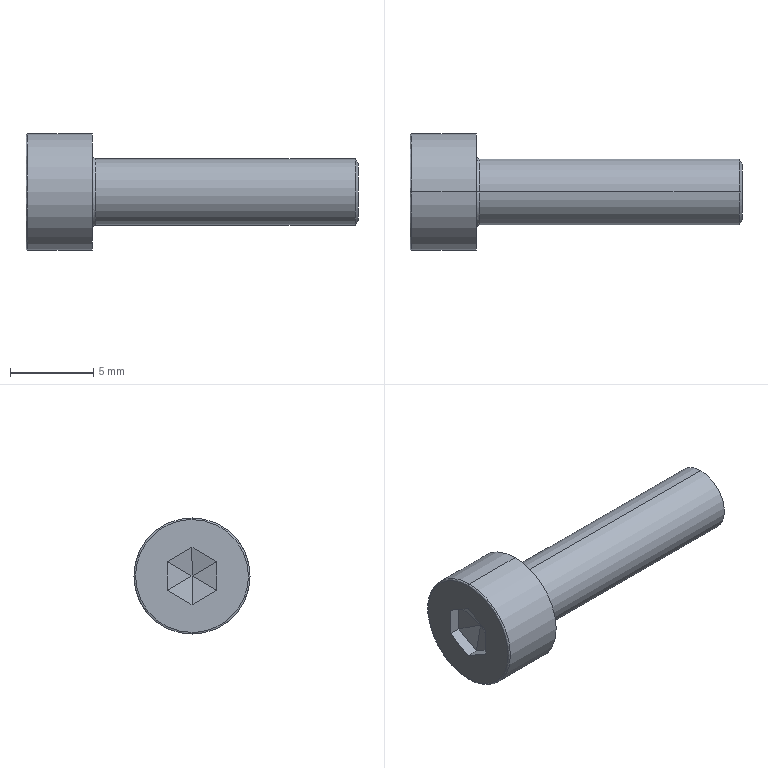Part | SolidWorks | features BaseBody 1 | 1 solid | 25 faces | box 20 x 7 x 7 mm | volume 348.346 mm3 | plane 15 | spline 4 | cylinder 4 | cone 2 | commonest cylinder face diameters 4 x2 7 x2
STEP:
#1=CARTESIAN_POINT('',(4.2,0.,-2.));
#2=VERTEX_POINT('',#1);
#3=CARTESIAN_POINT('',(4.2,0.,2.));
#4=VERTEX_POINT('',#3);
#5=CARTESIAN_POINT('',(4.2,0.,0.));
#6=DIRECTION('',(1.,0.,0.));
#7=DIRECTION('',(0.,0.,1.));
#8=AXIS2_PLACEMENT_3D('',#5,#6,#7);
#9=CIRCLE('',#8,2.);
#10=EDGE_CURVE('',#2,#4,#9,.T.);
#11=ORIENTED_EDGE('',*,*,#10,.F.);
#12=CARTESIAN_POINT('',(4.,0.,-2.2));
#13=VERTEX_POINT('',#12);
#14=CARTESIAN_POINT('',(4.2,0.,-2.2));
#15=DIRECTION('',(0.,-1.,0.));
#16=DIRECTION('',(0.,0.,-1.));
#17=AXIS2_PLACEMENT_3D('',#14,#15,#16);
#18=CIRCLE('',#17,0.2);
#19=EDGE_CURVE('',#2,#13,#18,.T.);
#20=ORIENTED_EDGE('',*,*,#19,.T.);
#21=CARTESIAN_POINT('',(4.,0.,2.2));
#22=VERTEX_POINT('',#21);
#23=CARTESIAN_POINT('',(4.,0.,2.2));
#24=CARTESIAN_POINT('',(4.,0.14,2.2));
#25=CARTESIAN_POINT('',(4.,0.3462,2.181));
#26=CARTESIAN_POINT('',(4.,0.5802,2.124));
#27=CARTESIAN_POINT('',(4.,0.6955,2.088));
#28=CARTESIAN_POINT('',(4.,0.7446,2.07));
#29=CARTESIAN_POINT('',(4.,0.7773,2.058));
#30=CARTESIAN_POINT('',(4.,0.7921,2.053));
#31=CARTESIAN_POINT('',(4.,1.093,1.934));
#32=CARTESIAN_POINT('',(4.,1.341,1.771));
#33=CARTESIAN_POINT('',(4.,1.663,1.448));
#34=CARTESIAN_POINT('',(4.,1.805,1.274));
#35=CARTESIAN_POINT('',(4.,1.937,1.049));
#36=CARTESIAN_POINT('',(4.,1.994,0.9314));
#37=CARTESIAN_POINT('',(4.,2.017,0.8797));
#38=CARTESIAN_POINT('',(4.,2.031,0.8449));
#39=CARTESIAN_POINT('',(4.,2.039,0.8261));
#40=CARTESIAN_POINT('',(4.,2.149,0.5493));
#41=CARTESIAN_POINT('',(4.,2.2,0.2801));
#42=CARTESIAN_POINT('',(4.,2.2,-0.1401));
#43=CARTESIAN_POINT('',(4.,2.181,-0.3463));
#44=CARTESIAN_POINT('',(4.,2.124,-0.5803));
#45=CARTESIAN_POINT('',(4.,2.088,-0.6956));
#46=CARTESIAN_POINT('',(4.,2.07,-0.7447));
#47=CARTESIAN_POINT('',(4.,2.058,-0.7773));
#48=CARTESIAN_POINT('',(4.,2.053,-0.7921));
#49=CARTESIAN_POINT('',(4.,1.934,-1.093));
#50=CARTESIAN_POINT('',(4.,1.771,-1.341));
#51=CARTESIAN_POINT('',(4.,1.448,-1.663));
#52=CARTESIAN_POINT('',(4.,1.274,-1.805));
#53=CARTESIAN_POINT('',(4.,1.049,-1.937));
#54=CARTESIAN_POINT('',(4.,0.9314,-1.994));
#55=CARTESIAN_POINT('',(4.,0.8797,-2.017));
#56=CARTESIAN_POINT('',(4.,0.8449,-2.031));
#57=CARTESIAN_POINT('',(4.,0.8261,-2.039));
#58=CARTESIAN_POINT('',(4.,0.5493,-2.149));
#59=CARTESIAN_POINT('',(4.,0.2801,-2.2));
#60=CARTESIAN_POINT('',(4.,0.,-2.2));
#61=B_SPLINE_CURVE_WITH_KNOTS('',3,(#23,#24,#25,#26,#27,#28,#29,#30,#31,#32,#33,#34,#35,#36,#37,#38,#39,#40,#41,#42,#43,#44,#45,#46,#47,#48,#49,#50,#51,#52,#53,#54,#55,#56,#57,#58,#59,#60),.UNSPECIFIED.,.F.,.F.,(4,1,1,1,2,2,2,1,1,1,2,2,2,1,1,1,2,2,2,1,1,1,2,2,4),(0.,0.03125,0.04688,0.05469,0.05859,0.0625,0.125,0.1563,0.1719,0.1797,0.1836,0.1875,0.25,0.2813,0.2969,0.3047,0.3086,0.3125,0.375,0.4062,0.4219,0.4297,0.4336,0.4375,0.5),.UNSPECIFIED.);
#62=EDGE_CURVE('',#22,#13,#61,.T.);
#63=ORIENTED_EDGE('',*,*,#62,.F.);
#64=CARTESIAN_POINT('',(4.2,0.,2.2));
#65=DIRECTION('',(0.,1.,0.));
#66=DIRECTION('',(0.,0.,1.));
#67=AXIS2_PLACEMENT_3D('',#64,#65,#66);
#68=CIRCLE('',#67,0.2);
#69=EDGE_CURVE('',#4,#22,#68,.T.);
#70=ORIENTED_EDGE('',*,*,#69,.F.);
#71=EDGE_LOOP('',(#11,#20,#63,#70));
#72=FACE_OUTER_BOUND('',#71,.T.);
#73=CARTESIAN_POINT('',(4.2,0.,2.));
#74=CARTESIAN_POINT('',(4.2,4.,2.));
#75=CARTESIAN_POINT('',(4.2,4.,-2.));
#76=CARTESIAN_POINT('',(4.2,0.,-2.));
#77=CARTESIAN_POINT('',(4.083,0.,2.));
#78=CARTESIAN_POINT('',(4.083,4.,2.));
#79=CARTESIAN_POINT('',(4.083,4.,-2.));
#80=CARTESIAN_POINT('',(4.083,0.,-2.));
#81=CARTESIAN_POINT('',(4.,0.,2.083));
#82=CARTESIAN_POINT('',(4.,4.166,2.083));
#83=CARTESIAN_POINT('',(4.,4.166,-2.083));
#84=CARTESIAN_POINT('',(4.,0.,-2.083));
#85=CARTESIAN_POINT('',(4.,0.,2.2));
#86=CARTESIAN_POINT('',(4.,4.4,2.2));
#87=CARTESIAN_POINT('',(4.,4.4,-2.2));
#88=CARTESIAN_POINT('',(4.,0.,-2.2));
#89=(BOUNDED_SURFACE()B_SPLINE_SURFACE(3,3,((#73,#74,#75,#76),(#77,#78,#79,#80),(#81,#82,#83,#84),(#85,#86,#87,#88)),.UNSPECIFIED.,.F.,.F.,.F.)B_SPLINE_SURFACE_WITH_KNOTS((4,4),(4,4),(0.,1.),(0.,1.),.UNSPECIFIED.)GEOMETRIC_REPRESENTATION_ITEM()RATIONAL_B_SPLINE_SURFACE(((1.,0.3333,0.3333,1.),(0.8047,0.2682,0.2682,0.8047),(0.8047,0.2682,0.2682,0.8047),(1.,0.3333,0.3333,1.)))REPRESENTATION_ITEM('')SURFACE());
#90=ADVANCED_FACE('',(#72),#89,.F.);
#91=CARTESIAN_POINT('',(0.1,0.,3.5));
#92=VERTEX_POINT('',#91);
#93=CARTESIAN_POINT('',(0.1,0.,-3.5));
#94=VERTEX_POINT('',#93);
#95=CARTESIAN_POINT('',(0.1,0.,0.));
#96=DIRECTION('',(1.,0.,0.));
#97=DIRECTION('',(0.,0.,1.));
#98=AXIS2_PLACEMENT_3D('',#95,#96,#97);
#99=CIRCLE('',#98,3.5);
#100=EDGE_CURVE('',#92,#94,#99,.T.);
#101=ORIENTED_EDGE('',*,*,#100,.F.);
#102=CARTESIAN_POINT('',(0.,0.,3.4));
#103=VERTEX_POINT('',#102);
#104=CARTESIAN_POINT('',(0.1,0.,3.4));
#105=DIRECTION('',(0.,-1.,0.));
#106=DIRECTION('',(0.,0.,1.));
#107=AXIS2_PLACEMENT_3D('',#104,#105,#106);
#108=CIRCLE('',#107,0.1);
#109=EDGE_CURVE('',#92,#103,#108,.T.);
#110=ORIENTED_EDGE('',*,*,#109,.T.);
#111=CARTESIAN_POINT('',(0.,0.,-3.4));
#112=VERTEX_POINT('',#111);
#113=CARTESIAN_POINT('',(0.,0.,3.4));
#114=CARTESIAN_POINT('',(0.,-6.8,3.4));
#115=CARTESIAN_POINT('',(0.,-6.8,-3.4));
#116=CARTESIAN_POINT('',(0.,0.,-3.4));
#117=(BOUNDED_CURVE()B_SPLINE_CURVE(3,(#113,#114,#115,#116),.UNSPECIFIED.,.F.,.F.)B_SPLINE_CURVE_WITH_KNOTS((4,4),(0.5,1.),.UNSPECIFIED.)CURVE()GEOMETRIC_REPRESENTATION_ITEM()RATIONAL_B_SPLINE_CURVE((1.,0.3333,0.3333,1.))REPRESENTATION_ITEM(''));
#118=EDGE_CURVE('',#103,#112,#117,.T.);
#119=ORIENTED_EDGE('',*,*,#118,.T.);
#120=CARTESIAN_POINT('',(0.1,0.,-3.4));
#121=DIRECTION('',(0.,1.,0.));
#122=DIRECTION('',(0.,0.,-1.));
#123=AXIS2_PLACEMENT_3D('',#120,#121,#122);
#124=CIRCLE('',#123,0.1);
#125=EDGE_CURVE('',#94,#112,#124,.T.);
#126=ORIENTED_EDGE('',*,*,#125,.F.);
#127=EDGE_LOOP('',(#101,#110,#119,#126));
#128=FACE_OUTER_BOUND('',#127,.T.);
#129=CARTESIAN_POINT('',(0.1,0.,3.5));
#130=CARTESIAN_POINT('',(0.1,-7.,3.5));
#131=CARTESIAN_POINT('',(0.1,-7.,-3.5));
#132=CARTESIAN_POINT('',(0.1,0.,-3.5));
#133=CARTESIAN_POINT('',(0.04142,0.,3.5));
#134=CARTESIAN_POINT('',(0.04142,-7.,3.5));
#135=CARTESIAN_POINT('',(0.04142,-7.,-3.5));
#136=CARTESIAN_POINT('',(0.04142,0.,-3.5));
#137=CARTESIAN_POINT('',(0.,0.,3.459));
#138=CARTESIAN_POINT('',(0.,-6.917,3.459));
#139=CARTESIAN_POINT('',(0.,-6.917,-3.459));
#140=CARTESIAN_POINT('',(0.,0.,-3.459));
#141=CARTESIAN_POINT('',(0.,0.,3.4));
#142=CARTESIAN_POINT('',(0.,-6.8,3.4));
#143=CARTESIAN_POINT('',(0.,-6.8,-3.4));
#144=CARTESIAN_POINT('',(0.,0.,-3.4));
#145=(BOUNDED_SURFACE()B_SPLINE_SURFACE(3,3,((#129,#130,#131,#132),(#133,#134,#135,#136),(#137,#138,#139,#140),(#141,#142,#143,#144)),.UNSPECIFIED.,.F.,.F.,.F.)B_SPLINE_SURFACE_WITH_KNOTS((4,4),(4,4),(0.,1.),(0.,1.),.UNSPECIFIED.)GEOMETRIC_REPRESENTATION_ITEM()RATIONAL_B_SPLINE_SURFACE(((1.,0.3333,0.3333,1.),(0.8047,0.2682,0.2682,0.8047),(0.8047,0.2682,0.2682,0.8047),(1.,0.3333,0.3333,1.)))REPRESENTATION_ITEM('')SURFACE());
#146=ADVANCED_FACE('',(#128),#145,.T.);
#147=CARTESIAN_POINT('',(19.825,0.,2.));
#148=VERTEX_POINT('',#147);
#149=CARTESIAN_POINT('',(19.825,0.,-2.));
#150=VERTEX_POINT('',#149);
#151=CARTESIAN_POINT('',(19.825,0.,0.));
#152=DIRECTION('',(-1.,0.,0.));
#153=DIRECTION('',(0.,0.,1.));
#154=AXIS2_PLACEMENT_3D('',#151,#152,#153);
#155=CIRCLE('',#154,2.);
#156=EDGE_CURVE('',#148,#150,#155,.T.);
#157=ORIENTED_EDGE('',*,*,#156,.T.);
#158=CARTESIAN_POINT('',(0.,0.,-2.));
#159=DIRECTION('',(-1.,0.,0.));
#160=VECTOR('',#159,1000.);
#161=LINE('',#158,#160);
#162=EDGE_CURVE('',#150,#2,#161,.T.);
#163=ORIENTED_EDGE('',*,*,#162,.T.);
#164=ORIENTED_EDGE('',*,*,#10,.T.);
#165=CARTESIAN_POINT('',(0.,0.,2.));
#166=DIRECTION('',(-1.,0.,0.));
#167=VECTOR('',#166,1000.);
#168=LINE('',#165,#167);
#169=EDGE_CURVE('',#148,#4,#168,.T.);
#170=ORIENTED_EDGE('',*,*,#169,.F.);
#171=EDGE_LOOP('',(#157,#163,#164,#170));
#172=FACE_OUTER_BOUND('',#171,.T.);
#173=CARTESIAN_POINT('',(0.,0.,0.));
#174=DIRECTION('',(-1.,0.,0.));
#175=DIRECTION('',(0.,0.,1.));
#176=AXIS2_PLACEMENT_3D('',#173,#174,#175);
#177=CYLINDRICAL_SURFACE('',#176,2.);
#178=ADVANCED_FACE('',(#172),#177,.T.);
#179=CARTESIAN_POINT('',(20.,0.,1.697));
#180=VERTEX_POINT('',#179);
#181=CARTESIAN_POINT('',(20.,0.,-1.697));
#182=VERTEX_POINT('',#181);
#183=CARTESIAN_POINT('',(20.,0.,0.));
#184=DIRECTION('',(-1.,0.,0.));
#185=DIRECTION('',(0.,0.,1.));
#186=AXIS2_PLACEMENT_3D('',#183,#184,#185);
#187=CIRCLE('',#186,1.697);
#188=EDGE_CURVE('',#180,#182,#187,.T.);
#189=ORIENTED_EDGE('',*,*,#188,.T.);
#190=CARTESIAN_POINT('',(19.825,0.,-2.));
#191=DIRECTION('',(-0.5,0.,-0.866));
#192=VECTOR('',#191,1000.);
#193=LINE('',#190,#192);
#194=EDGE_CURVE('',#182,#150,#193,.T.);
#195=ORIENTED_EDGE('',*,*,#194,.T.);
#196=ORIENTED_EDGE('',*,*,#156,.F.);
#197=CARTESIAN_POINT('',(19.825,0.,2.));
#198=DIRECTION('',(-0.5,0.,0.866));
#199=VECTOR('',#198,1000.);
#200=LINE('',#197,#199);
#201=EDGE_CURVE('',#180,#148,#200,.T.);
#202=ORIENTED_EDGE('',*,*,#201,.F.);
#203=EDGE_LOOP('',(#189,#195,#196,#202));
#204=FACE_OUTER_BOUND('',#203,.T.);
#205=CARTESIAN_POINT('',(19.825,0.,0.));
#206=DIRECTION('',(-1.,0.,0.));
#207=DIRECTION('',(0.,0.,1.));
#208=AXIS2_PLACEMENT_3D('',#205,#206,#207);
#209=CONICAL_SURFACE('',#208,2.,1.047);
#210=ADVANCED_FACE('',(#204),#209,.T.);
#211=CARTESIAN_POINT('',(4.,0.,3.5));
#212=VERTEX_POINT('',#211);
#213=CARTESIAN_POINT('',(4.,0.,-3.5));
#214=VERTEX_POINT('',#213);
#215=CARTESIAN_POINT('',(4.,0.,0.));
#216=DIRECTION('',(-1.,0.,0.));
#217=DIRECTION('',(0.,0.,1.));
#218=AXIS2_PLACEMENT_3D('',#215,#216,#217);
#219=CIRCLE('',#218,3.5);
#220=EDGE_CURVE('',#212,#214,#219,.T.);
#221=ORIENTED_EDGE('',*,*,#220,.T.);
#222=CARTESIAN_POINT('',(0.,0.,-3.5));
#223=DIRECTION('',(-1.,0.,0.));
#224=VECTOR('',#223,1000.);
#225=LINE('',#222,#224);
#226=EDGE_CURVE('',#214,#94,#225,.T.);
#227=ORIENTED_EDGE('',*,*,#226,.T.);
#228=CARTESIAN_POINT('',(0.1,0.,0.));
#229=DIRECTION('',(1.,0.,0.));
#230=DIRECTION('',(0.,0.,1.));
#231=AXIS2_PLACEMENT_3D('',#228,#229,#230);
#232=CIRCLE('',#231,3.5);
#233=EDGE_CURVE('',#94,#92,#232,.T.);
#234=ORIENTED_EDGE('',*,*,#233,.T.);
#235=CARTESIAN_POINT('',(0.,0.,3.5));
#236=DIRECTION('',(-1.,0.,0.));
#237=VECTOR('',#236,1000.);
#238=LINE('',#235,#237);
#239=EDGE_CURVE('',#212,#92,#238,.T.);
#240=ORIENTED_EDGE('',*,*,#239,.F.);
#241=EDGE_LOOP('',(#221,#227,#234,#240));
#242=FACE_OUTER_BOUND('',#241,.T.);
#243=CARTESIAN_POINT('',(0.,0.,0.));
#244=DIRECTION('',(-1.,0.,0.));
#245=DIRECTION('',(0.,0.,1.));
#246=AXIS2_PLACEMENT_3D('',#243,#244,#245);
#247=CYLINDRICAL_SURFACE('',#246,3.5);
#248=ADVANCED_FACE('',(#242),#247,.T.);
#249=ORIENTED_EDGE('',*,*,#162,.F.);
#250=CARTESIAN_POINT('',(19.825,0.,0.));
#251=DIRECTION('',(-1.,0.,0.));
#252=DIRECTION('',(0.,0.,1.));
#253=AXIS2_PLACEMENT_3D('',#250,#251,#252);
#254=CIRCLE('',#253,2.);
#255=EDGE_CURVE('',#150,#148,#254,.T.);
#256=ORIENTED_EDGE('',*,*,#255,.T.);
#257=ORIENTED_EDGE('',*,*,#169,.T.);
#258=CARTESIAN_POINT('',(4.2,0.,0.));
#259=DIRECTION('',(1.,0.,0.));
#260=DIRECTION('',(0.,0.,1.));
#261=AXIS2_PLACEMENT_3D('',#258,#259,#260);
#262=CIRCLE('',#261,2.);
#263=EDGE_CURVE('',#4,#2,#262,.T.);
#264=ORIENTED_EDGE('',*,*,#263,.T.);
#265=EDGE_LOOP('',(#249,#256,#257,#264));
#266=FACE_OUTER_BOUND('',#265,.T.);
#267=CARTESIAN_POINT('',(0.,0.,0.));
#268=DIRECTION('',(-1.,0.,0.));
#269=DIRECTION('',(0.,0.,1.));
#270=AXIS2_PLACEMENT_3D('',#267,#268,#269);
#271=CYLINDRICAL_SURFACE('',#270,2.);
#272=ADVANCED_FACE('',(#266),#271,.T.);
#273=ORIENTED_EDGE('',*,*,#194,.F.);
#274=CARTESIAN_POINT('',(20.,0.,0.));
#275=DIRECTION('',(-1.,0.,0.));
#276=DIRECTION('',(0.,0.,1.));
#277=AXIS2_PLACEMENT_3D('',#274,#275,#276);
#278=CIRCLE('',#277,1.697);
#279=EDGE_CURVE('',#182,#180,#278,.T.);
#280=ORIENTED_EDGE('',*,*,#279,.T.);
#281=ORIENTED_EDGE('',*,*,#201,.T.);
#282=ORIENTED_EDGE('',*,*,#255,.F.);
#283=EDGE_LOOP('',(#273,#280,#281,#282));
#284=FACE_OUTER_BOUND('',#283,.T.);
#285=CARTESIAN_POINT('',(19.825,0.,0.));
#286=DIRECTION('',(-1.,0.,0.));
#287=DIRECTION('',(0.,0.,1.));
#288=AXIS2_PLACEMENT_3D('',#285,#286,#287);
#289=CONICAL_SURFACE('',#288,2.,1.047);
#290=ADVANCED_FACE('',(#284),#289,.T.);
#291=ORIENTED_EDGE('',*,*,#19,.F.);
#292=ORIENTED_EDGE('',*,*,#263,.F.);
#293=ORIENTED_EDGE('',*,*,#69,.T.);
#294=CARTESIAN_POINT('',(4.,0.,-2.2));
#295=CARTESIAN_POINT('',(4.,-0.1401,-2.2));
#296=CARTESIAN_POINT('',(4.,-0.3463,-2.181));
#297=CARTESIAN_POINT('',(4.,-0.5803,-2.124));
#298=CARTESIAN_POINT('',(4.,-0.6956,-2.088));
#299=CARTESIAN_POINT('',(4.,-0.7447,-2.07));
#300=CARTESIAN_POINT('',(4.,-0.7773,-2.058));
#301=CARTESIAN_POINT('',(4.,-0.7921,-2.053));
#302=CARTESIAN_POINT('',(4.,-1.093,-1.934));
#303=CARTESIAN_POINT('',(4.,-1.341,-1.771));
#304=CARTESIAN_POINT('',(4.,-1.663,-1.448));
#305=CARTESIAN_POINT('',(4.,-1.805,-1.274));
#306=CARTESIAN_POINT('',(4.,-1.937,-1.049));
#307=CARTESIAN_POINT('',(4.,-1.994,-0.9314));
#308=CARTESIAN_POINT('',(4.,-2.017,-0.8797));
#309=CARTESIAN_POINT('',(4.,-2.031,-0.8449));
#310=CARTESIAN_POINT('',(4.,-2.039,-0.8261));
#311=CARTESIAN_POINT('',(4.,-2.149,-0.5493));
#312=CARTESIAN_POINT('',(4.,-2.2,-0.2801));
#313=CARTESIAN_POINT('',(4.,-2.2,0.1401));
#314=CARTESIAN_POINT('',(4.,-2.181,0.3463));
#315=CARTESIAN_POINT('',(4.,-2.124,0.5803));
#316=CARTESIAN_POINT('',(4.,-2.088,0.6956));
#317=CARTESIAN_POINT('',(4.,-2.07,0.7447));
#318=CARTESIAN_POINT('',(4.,-2.058,0.7773));
#319=CARTESIAN_POINT('',(4.,-2.053,0.7921));
#320=CARTESIAN_POINT('',(4.,-1.934,1.093));
#321=CARTESIAN_POINT('',(4.,-1.771,1.341));
#322=CARTESIAN_POINT('',(4.,-1.448,1.663));
#323=CARTESIAN_POINT('',(4.,-1.274,1.805));
#324=CARTESIAN_POINT('',(4.,-1.049,1.937));
#325=CARTESIAN_POINT('',(4.,-0.9314,1.994));
#326=CARTESIAN_POINT('',(4.,-0.8797,2.017));
#327=CARTESIAN_POINT('',(4.,-0.8449,2.031));
#328=CARTESIAN_POINT('',(4.,-0.8261,2.039));
#329=CARTESIAN_POINT('',(4.,-0.5495,2.149));
#330=CARTESIAN_POINT('',(4.,-0.2796,2.2));
#331=CARTESIAN_POINT('',(4.,0.,2.2));
#332=B_SPLINE_CURVE_WITH_KNOTS('',3,(#294,#295,#296,#297,#298,#299,#300,#301,#302,#303,#304,#305,#306,#307,#308,#309,#310,#311,#312,#313,#314,#315,#316,#317,#318,#319,#320,#321,#322,#323,#324,#325,#326,#327,#328,#329,#330,#331),.UNSPECIFIED.,.F.,.F.,(4,1,1,1,2,2,2,1,1,1,2,2,2,1,1,1,2,2,2,1,1,1,2,2,4),(0.5,0.5312,0.5469,0.5547,0.5586,0.5625,0.625,0.6562,0.6719,0.6797,0.6836,0.6875,0.75,0.7812,0.7969,0.8047,0.8086,0.8125,0.875,0.9062,0.9219,0.9297,0.9336,0.9375,1.),.UNSPECIFIED.);
#333=EDGE_CURVE('',#13,#22,#332,.T.);
#334=ORIENTED_EDGE('',*,*,#333,.F.);
#335=EDGE_LOOP('',(#291,#292,#293,#334));
#336=FACE_OUTER_BOUND('',#335,.T.);
#337=CARTESIAN_POINT('',(4.2,0.,-2.));
#338=CARTESIAN_POINT('',(4.2,-4.,-2.));
#339=CARTESIAN_POINT('',(4.2,-4.,2.));
#340=CARTESIAN_POINT('',(4.2,0.,2.));
#341=CARTESIAN_POINT('',(4.083,0.,-2.));
#342=CARTESIAN_POINT('',(4.083,-4.,-2.));
#343=CARTESIAN_POINT('',(4.083,-4.,2.));
#344=CARTESIAN_POINT('',(4.083,0.,2.));
#345=CARTESIAN_POINT('',(4.,0.,-2.083));
#346=CARTESIAN_POINT('',(4.,-4.166,-2.083));
#347=CARTESIAN_POINT('',(4.,-4.166,2.083));
#348=CARTESIAN_POINT('',(4.,0.,2.083));
#349=CARTESIAN_POINT('',(4.,0.,-2.2));
#350=CARTESIAN_POINT('',(4.,-4.4,-2.2));
#351=CARTESIAN_POINT('',(4.,-4.4,2.2));
#352=CARTESIAN_POINT('',(4.,0.,2.2));
#353=(BOUNDED_SURFACE()B_SPLINE_SURFACE(3,3,((#337,#338,#339,#340),(#341,#342,#343,#344),(#345,#346,#347,#348),(#349,#350,#351,#352)),.UNSPECIFIED.,.F.,.F.,.F.)B_SPLINE_SURFACE_WITH_KNOTS((4,4),(4,4),(0.,1.),(0.,1.),.UNSPECIFIED.)GEOMETRIC_REPRESENTATION_ITEM()RATIONAL_B_SPLINE_SURFACE(((1.,0.3333,0.3333,1.),(0.8047,0.2682,0.2682,0.8047),(0.8047,0.2682,0.2682,0.8047),(1.,0.3333,0.3333,1.)))REPRESENTATION_ITEM('')SURFACE());
#354=ADVANCED_FACE('',(#336),#353,.F.);
#355=ORIENTED_EDGE('',*,*,#188,.F.);
#356=ORIENTED_EDGE('',*,*,#279,.F.);
#357=EDGE_LOOP('',(#355,#356));
#358=FACE_OUTER_BOUND('',#357,.T.);
#359=CARTESIAN_POINT('',(20.,2.,0.));
#360=DIRECTION('',(-1.,0.,0.));
#361=DIRECTION('',(0.,0.,1.));
#362=AXIS2_PLACEMENT_3D('',#359,#360,#361);
#363=PLANE('',#362);
#364=ADVANCED_FACE('',(#358),#363,.F.);
#365=ORIENTED_EDGE('',*,*,#62,.T.);
#366=ORIENTED_EDGE('',*,*,#333,.T.);
#367=EDGE_LOOP('',(#365,#366));
#368=FACE_BOUND('',#367,.T.);
#369=ORIENTED_EDGE('',*,*,#220,.F.);
#370=CARTESIAN_POINT('',(4.,0.,0.));
#371=DIRECTION('',(-1.,0.,0.));
#372=DIRECTION('',(0.,0.,1.));
#373=AXIS2_PLACEMENT_3D('',#370,#371,#372);
#374=CIRCLE('',#373,3.5);
#375=EDGE_CURVE('',#214,#212,#374,.T.);
#376=ORIENTED_EDGE('',*,*,#375,.F.);
#377=EDGE_LOOP('',(#369,#376));
#378=FACE_OUTER_BOUND('',#377,.T.);
#379=CARTESIAN_POINT('',(4.,3.5,0.));
#380=DIRECTION('',(-1.,0.,0.));
#381=DIRECTION('',(0.,0.,1.));
#382=AXIS2_PLACEMENT_3D('',#379,#380,#381);
#383=PLANE('',#382);
#384=ADVANCED_FACE('',(#368,#378),#383,.F.);
#385=ORIENTED_EDGE('',*,*,#226,.F.);
#386=ORIENTED_EDGE('',*,*,#375,.T.);
#387=ORIENTED_EDGE('',*,*,#239,.T.);
#388=ORIENTED_EDGE('',*,*,#100,.T.);
#389=EDGE_LOOP('',(#385,#386,#387,#388));
#390=FACE_OUTER_BOUND('',#389,.T.);
#391=CARTESIAN_POINT('',(0.,0.,0.));
#392=DIRECTION('',(-1.,0.,0.));
#393=DIRECTION('',(0.,0.,1.));
#394=AXIS2_PLACEMENT_3D('',#391,#392,#393);
#395=CYLINDRICAL_SURFACE('',#394,3.5);
#396=ADVANCED_FACE('',(#390),#395,.T.);
#397=ORIENTED_EDGE('',*,*,#109,.F.);
#398=ORIENTED_EDGE('',*,*,#233,.F.);
#399=ORIENTED_EDGE('',*,*,#125,.T.);
#400=CARTESIAN_POINT('',(0.,0.,-3.4));
#401=CARTESIAN_POINT('',(0.,6.8,-3.4));
#402=CARTESIAN_POINT('',(0.,6.8,3.4));
#403=CARTESIAN_POINT('',(0.,0.,3.4));
#404=(BOUNDED_CURVE()B_SPLINE_CURVE(3,(#400,#401,#402,#403),.UNSPECIFIED.,.F.,.F.)B_SPLINE_CURVE_WITH_KNOTS((4,4),(0.,0.5),.UNSPECIFIED.)CURVE()GEOMETRIC_REPRESENTATION_ITEM()RATIONAL_B_SPLINE_CURVE((1.,0.3333,0.3333,1.))REPRESENTATION_ITEM(''));
#405=EDGE_CURVE('',#112,#103,#404,.T.);
#406=ORIENTED_EDGE('',*,*,#405,.T.);
#407=EDGE_LOOP('',(#397,#398,#399,#406));
#408=FACE_OUTER_BOUND('',#407,.T.);
#409=CARTESIAN_POINT('',(0.1,0.,-3.5));
#410=CARTESIAN_POINT('',(0.1,7.,-3.5));
#411=CARTESIAN_POINT('',(0.1,7.,3.5));
#412=CARTESIAN_POINT('',(0.1,0.,3.5));
#413=CARTESIAN_POINT('',(0.04142,0.,-3.5));
#414=CARTESIAN_POINT('',(0.04142,7.,-3.5));
#415=CARTESIAN_POINT('',(0.04142,7.,3.5));
#416=CARTESIAN_POINT('',(0.04142,0.,3.5));
#417=CARTESIAN_POINT('',(0.,0.,-3.459));
#418=CARTESIAN_POINT('',(0.,6.917,-3.459));
#419=CARTESIAN_POINT('',(0.,6.917,3.459));
#420=CARTESIAN_POINT('',(0.,0.,3.459));
#421=CARTESIAN_POINT('',(0.,0.,-3.4));
#422=CARTESIAN_POINT('',(0.,6.8,-3.4));
#423=CARTESIAN_POINT('',(0.,6.8,3.4));
#424=CARTESIAN_POINT('',(0.,0.,3.4));
#425=(BOUNDED_SURFACE()B_SPLINE_SURFACE(3,3,((#409,#410,#411,#412),(#413,#414,#415,#416),(#417,#418,#419,#420),(#421,#422,#423,#424)),.UNSPECIFIED.,.F.,.F.,.F.)B_SPLINE_SURFACE_WITH_KNOTS((4,4),(4,4),(0.,1.),(0.,1.),.UNSPECIFIED.)GEOMETRIC_REPRESENTATION_ITEM()RATIONAL_B_SPLINE_SURFACE(((1.,0.3333,0.3333,1.),(0.8047,0.2682,0.2682,0.8047),(0.8047,0.2682,0.2682,0.8047),(1.,0.3333,0.3333,1.)))REPRESENTATION_ITEM('')SURFACE());
#426=ADVANCED_FACE('',(#408),#425,.T.);
#427=CARTESIAN_POINT('',(0.,-1.5,0.866));
#428=VERTEX_POINT('',#427);
#429=CARTESIAN_POINT('',(0.,0.,1.732));
#430=VERTEX_POINT('',#429);
#431=CARTESIAN_POINT('',(0.,-1.5,0.866));
#432=DIRECTION('',(0.,0.866,0.5));
#433=VECTOR('',#432,1000.);
#434=LINE('',#431,#433);
#435=EDGE_CURVE('',#428,#430,#434,.T.);
#436=ORIENTED_EDGE('',*,*,#435,.F.);
#437=CARTESIAN_POINT('',(0.,-1.5,-0.866));
#438=VERTEX_POINT('',#437);
#439=CARTESIAN_POINT('',(0.,-1.5,0.));
#440=DIRECTION('',(0.,0.,1.));
#441=VECTOR('',#440,1000.);
#442=LINE('',#439,#441);
#443=EDGE_CURVE('',#438,#428,#442,.T.);
#444=ORIENTED_EDGE('',*,*,#443,.F.);
#445=CARTESIAN_POINT('',(0.,0.,-1.732));
#446=VERTEX_POINT('',#445);
#447=CARTESIAN_POINT('',(0.,0.,-1.732));
#448=DIRECTION('',(0.,-0.866,0.5));
#449=VECTOR('',#448,1000.);
#450=LINE('',#447,#449);
#451=EDGE_CURVE('',#446,#438,#450,.T.);
#452=ORIENTED_EDGE('',*,*,#451,.F.);
#453=CARTESIAN_POINT('',(0.,1.5,-0.866));
#454=VERTEX_POINT('',#453);
#455=CARTESIAN_POINT('',(0.,1.5,-0.866));
#456=DIRECTION('',(0.,-0.866,-0.5));
#457=VECTOR('',#456,1000.);
#458=LINE('',#455,#457);
#459=EDGE_CURVE('',#454,#446,#458,.T.);
#460=ORIENTED_EDGE('',*,*,#459,.F.);
#461=CARTESIAN_POINT('',(0.,1.5,0.866));
#462=VERTEX_POINT('',#461);
#463=CARTESIAN_POINT('',(0.,1.5,0.));
#464=DIRECTION('',(0.,0.,-1.));
#465=VECTOR('',#464,1000.);
#466=LINE('',#463,#465);
#467=EDGE_CURVE('',#462,#454,#466,.T.);
#468=ORIENTED_EDGE('',*,*,#467,.F.);
#469=CARTESIAN_POINT('',(0.,0.,1.732));
#470=DIRECTION('',(0.,0.866,-0.5));
#471=VECTOR('',#470,1000.);
#472=LINE('',#469,#471);
#473=EDGE_CURVE('',#430,#462,#472,.T.);
#474=ORIENTED_EDGE('',*,*,#473,.F.);
#475=EDGE_LOOP('',(#436,#444,#452,#460,#468,#474));
#476=FACE_BOUND('',#475,.T.);
#477=ORIENTED_EDGE('',*,*,#405,.F.);
#478=ORIENTED_EDGE('',*,*,#118,.F.);
#479=EDGE_LOOP('',(#477,#478));
#480=FACE_OUTER_BOUND('',#479,.T.);
#481=CARTESIAN_POINT('',(0.,0.,0.));
#482=DIRECTION('',(1.,0.,0.));
#483=DIRECTION('',(0.,0.,-1.));
#484=AXIS2_PLACEMENT_3D('',#481,#482,#483);
#485=PLANE('',#484);
#486=ADVANCED_FACE('',(#476,#480),#485,.F.);
#487=CARTESIAN_POINT('',(0.7,1.5,0.866));
#488=VERTEX_POINT('',#487);
#489=CARTESIAN_POINT('',(0.7,1.5,0.866));
#490=DIRECTION('',(-1.,0.,0.));
#491=VECTOR('',#490,1000.);
#492=LINE('',#489,#491);
#493=EDGE_CURVE('',#488,#462,#492,.T.);
#494=ORIENTED_EDGE('',*,*,#493,.F.);
#495=CARTESIAN_POINT('',(0.7,0.,1.732));
#496=VERTEX_POINT('',#495);
#497=CARTESIAN_POINT('',(0.7,0.,1.732));
#498=DIRECTION('',(0.,0.866,-0.5));
#499=VECTOR('',#498,1000.);
#500=LINE('',#497,#499);
#501=EDGE_CURVE('',#496,#488,#500,.T.);
#502=ORIENTED_EDGE('',*,*,#501,.F.);
#503=CARTESIAN_POINT('',(0.7,0.,1.732));
#504=DIRECTION('',(1.,0.,0.));
#505=VECTOR('',#504,1000.);
#506=LINE('',#503,#505);
#507=EDGE_CURVE('',#430,#496,#506,.T.);
#508=ORIENTED_EDGE('',*,*,#507,.F.);
#509=ORIENTED_EDGE('',*,*,#473,.T.);
#510=EDGE_LOOP('',(#494,#502,#508,#509));
#511=FACE_OUTER_BOUND('',#510,.T.);
#512=CARTESIAN_POINT('',(0.7,0.,1.732));
#513=DIRECTION('',(0.,0.5,0.866));
#514=DIRECTION('',(0.,-0.866,0.5));
#515=AXIS2_PLACEMENT_3D('',#512,#513,#514);
#516=PLANE('',#515);
#517=ADVANCED_FACE('',(#511),#516,.F.);
#518=ORIENTED_EDGE('',*,*,#507,.T.);
#519=CARTESIAN_POINT('',(0.7,-1.5,0.866));
#520=VERTEX_POINT('',#519);
#521=CARTESIAN_POINT('',(0.7,-1.5,0.866));
#522=DIRECTION('',(0.,0.866,0.5));
#523=VECTOR('',#522,1000.);
#524=LINE('',#521,#523);
#525=EDGE_CURVE('',#520,#496,#524,.T.);
#526=ORIENTED_EDGE('',*,*,#525,.F.);
#527=CARTESIAN_POINT('',(0.7,-1.5,0.866));
#528=DIRECTION('',(1.,0.,0.));
#529=VECTOR('',#528,1000.);
#530=LINE('',#527,#529);
#531=EDGE_CURVE('',#428,#520,#530,.T.);
#532=ORIENTED_EDGE('',*,*,#531,.F.);
#533=ORIENTED_EDGE('',*,*,#435,.T.);
#534=EDGE_LOOP('',(#518,#526,#532,#533));
#535=FACE_OUTER_BOUND('',#534,.T.);
#536=CARTESIAN_POINT('',(0.7,-1.5,0.866));
#537=DIRECTION('',(0.,-0.5,0.866));
#538=DIRECTION('',(0.,-0.866,-0.5));
#539=AXIS2_PLACEMENT_3D('',#536,#537,#538);
#540=PLANE('',#539);
#541=ADVANCED_FACE('',(#535),#540,.F.);
#542=ORIENTED_EDGE('',*,*,#531,.T.);
#543=CARTESIAN_POINT('',(0.7,-1.5,-0.866));
#544=VERTEX_POINT('',#543);
#545=CARTESIAN_POINT('',(0.7,-1.5,0.866));
#546=DIRECTION('',(0.,0.,1.));
#547=VECTOR('',#546,1000.);
#548=LINE('',#545,#547);
#549=EDGE_CURVE('',#544,#520,#548,.T.);
#550=ORIENTED_EDGE('',*,*,#549,.F.);
#551=CARTESIAN_POINT('',(0.7,-1.5,-0.866));
#552=DIRECTION('',(1.,0.,0.));
#553=VECTOR('',#552,1000.);
#554=LINE('',#551,#553);
#555=EDGE_CURVE('',#438,#544,#554,.T.);
#556=ORIENTED_EDGE('',*,*,#555,.F.);
#557=ORIENTED_EDGE('',*,*,#443,.T.);
#558=EDGE_LOOP('',(#542,#550,#556,#557));
#559=FACE_OUTER_BOUND('',#558,.T.);
#560=CARTESIAN_POINT('',(0.7,-1.5,-0.866));
#561=DIRECTION('',(0.,-1.,0.));
#562=DIRECTION('',(0.,0.,-1.));
#563=AXIS2_PLACEMENT_3D('',#560,#561,#562);
#564=PLANE('',#563);
#565=ADVANCED_FACE('',(#559),#564,.F.);
#566=ORIENTED_EDGE('',*,*,#555,.T.);
#567=CARTESIAN_POINT('',(0.7,0.,-1.732));
#568=VERTEX_POINT('',#567);
#569=CARTESIAN_POINT('',(0.7,0.,-1.732));
#570=DIRECTION('',(0.,-0.866,0.5));
#571=VECTOR('',#570,1000.);
#572=LINE('',#569,#571);
#573=EDGE_CURVE('',#568,#544,#572,.T.);
#574=ORIENTED_EDGE('',*,*,#573,.F.);
#575=CARTESIAN_POINT('',(0.7,0.,-1.732));
#576=DIRECTION('',(1.,0.,0.));
#577=VECTOR('',#576,1000.);
#578=LINE('',#575,#577);
#579=EDGE_CURVE('',#446,#568,#578,.T.);
#580=ORIENTED_EDGE('',*,*,#579,.F.);
#581=ORIENTED_EDGE('',*,*,#451,.T.);
#582=EDGE_LOOP('',(#566,#574,#580,#581));
#583=FACE_OUTER_BOUND('',#582,.T.);
#584=CARTESIAN_POINT('',(0.7,0.,-1.732));
#585=DIRECTION('',(0.,-0.5,-0.866));
#586=DIRECTION('',(0.,0.866,-0.5));
#587=AXIS2_PLACEMENT_3D('',#584,#585,#586);
#588=PLANE('',#587);
#589=ADVANCED_FACE('',(#583),#588,.F.);
#590=ORIENTED_EDGE('',*,*,#579,.T.);
#591=CARTESIAN_POINT('',(0.7,1.5,-0.866));
#592=VERTEX_POINT('',#591);
#593=CARTESIAN_POINT('',(0.7,1.5,-0.866));
#594=DIRECTION('',(0.,-0.866,-0.5));
#595=VECTOR('',#594,1000.);
#596=LINE('',#593,#595);
#597=EDGE_CURVE('',#592,#568,#596,.T.);
#598=ORIENTED_EDGE('',*,*,#597,.F.);
#599=CARTESIAN_POINT('',(0.7,1.5,-0.866));
#600=DIRECTION('',(1.,0.,0.));
#601=VECTOR('',#600,1000.);
#602=LINE('',#599,#601);
#603=EDGE_CURVE('',#454,#592,#602,.T.);
#604=ORIENTED_EDGE('',*,*,#603,.F.);
#605=ORIENTED_EDGE('',*,*,#459,.T.);
#606=EDGE_LOOP('',(#590,#598,#604,#605));
#607=FACE_OUTER_BOUND('',#606,.T.);
#608=CARTESIAN_POINT('',(0.7,1.5,-0.866));
#609=DIRECTION('',(0.,0.5,-0.866));
#610=DIRECTION('',(0.,0.866,0.5));
#611=AXIS2_PLACEMENT_3D('',#608,#609,#610);
#612=PLANE('',#611);
#613=ADVANCED_FACE('',(#607),#612,.F.);
#614=ORIENTED_EDGE('',*,*,#603,.T.);
#615=CARTESIAN_POINT('',(0.7,1.5,-0.866));
#616=DIRECTION('',(0.,0.,-1.));
#617=VECTOR('',#616,1000.);
#618=LINE('',#615,#617);
#619=EDGE_CURVE('',#488,#592,#618,.T.);
#620=ORIENTED_EDGE('',*,*,#619,.F.);
#621=ORIENTED_EDGE('',*,*,#493,.T.);
#622=ORIENTED_EDGE('',*,*,#467,.T.);
#623=EDGE_LOOP('',(#614,#620,#621,#622));
#624=FACE_OUTER_BOUND('',#623,.T.);
#625=CARTESIAN_POINT('',(0.7,1.5,0.866));
#626=DIRECTION('',(0.,1.,0.));
#627=DIRECTION('',(0.,0.,1.));
#628=AXIS2_PLACEMENT_3D('',#625,#626,#627);
#629=PLANE('',#628);
#630=ADVANCED_FACE('',(#624),#629,.F.);
#631=CARTESIAN_POINT('',(1.067,0.,0.));
#632=VERTEX_POINT('',#631);
#633=CARTESIAN_POINT('',(0.8756,0.,0.9032));
#634=DIRECTION('',(-0.2072,0.,0.9783));
#635=VECTOR('',#634,1000.);
#636=LINE('',#633,#635);
#637=EDGE_CURVE('',#632,#496,#636,.T.);
#638=ORIENTED_EDGE('',*,*,#637,.T.);
#639=ORIENTED_EDGE('',*,*,#501,.T.);
#640=CARTESIAN_POINT('',(0.7,1.5,0.866));
#641=DIRECTION('',(0.2072,-0.8472,-0.4891));
#642=VECTOR('',#641,1000.);
#643=LINE('',#640,#642);
#644=EDGE_CURVE('',#488,#632,#643,.T.);
#645=ORIENTED_EDGE('',*,*,#644,.T.);
#646=EDGE_LOOP('',(#638,#639,#645));
#647=FACE_OUTER_BOUND('',#646,.T.);
#648=CARTESIAN_POINT('',(0.7,1.5,0.866));
#649=DIRECTION('',(-0.9714,-0.1188,-0.2058));
#650=DIRECTION('',(-0.2072,0.,0.9783));
#651=AXIS2_PLACEMENT_3D('',#648,#649,#650);
#652=PLANE('',#651);
#653=ADVANCED_FACE('',(#647),#652,.T.);
#654=CARTESIAN_POINT('',(1.067,0.,0.));
#655=DIRECTION('',(-0.2072,-0.8472,0.4891));
#656=VECTOR('',#655,1000.);
#657=LINE('',#654,#656);
#658=EDGE_CURVE('',#632,#520,#657,.T.);
#659=ORIENTED_EDGE('',*,*,#658,.T.);
#660=ORIENTED_EDGE('',*,*,#525,.T.);
#661=ORIENTED_EDGE('',*,*,#637,.F.);
#662=EDGE_LOOP('',(#659,#660,#661));
#663=FACE_OUTER_BOUND('',#662,.T.);
#664=CARTESIAN_POINT('',(0.7,0.,1.732));
#665=DIRECTION('',(-0.9714,0.1188,-0.2058));
#666=DIRECTION('',(-0.2072,0.,0.9783));
#667=AXIS2_PLACEMENT_3D('',#664,#665,#666);
#668=PLANE('',#667);
#669=ADVANCED_FACE('',(#663),#668,.T.);
#670=ORIENTED_EDGE('',*,*,#644,.F.);
#671=ORIENTED_EDGE('',*,*,#619,.T.);
#672=CARTESIAN_POINT('',(0.7,1.5,-0.866));
#673=DIRECTION('',(0.2072,-0.8472,0.4891));
#674=VECTOR('',#673,1000.);
#675=LINE('',#672,#674);
#676=EDGE_CURVE('',#592,#632,#675,.T.);
#677=ORIENTED_EDGE('',*,*,#676,.T.);
#678=EDGE_LOOP('',(#670,#671,#677));
#679=FACE_OUTER_BOUND('',#678,.T.);
#680=CARTESIAN_POINT('',(0.7,1.5,-0.866));
#681=DIRECTION('',(-0.9714,-0.2376,0.));
#682=DIRECTION('',(0.2376,-0.9714,0.));
#683=AXIS2_PLACEMENT_3D('',#680,#681,#682);
#684=PLANE('',#683);
#685=ADVANCED_FACE('',(#679),#684,.T.);
#686=CARTESIAN_POINT('',(1.067,0.,0.));
#687=DIRECTION('',(-0.2072,-0.8472,-0.4891));
#688=VECTOR('',#687,1000.);
#689=LINE('',#686,#688);
#690=EDGE_CURVE('',#632,#544,#689,.T.);
#691=ORIENTED_EDGE('',*,*,#690,.T.);
#692=ORIENTED_EDGE('',*,*,#549,.T.);
#693=ORIENTED_EDGE('',*,*,#658,.F.);
#694=EDGE_LOOP('',(#691,#692,#693));
#695=FACE_OUTER_BOUND('',#694,.T.);
#696=CARTESIAN_POINT('',(0.7,-1.5,0.866));
#697=DIRECTION('',(-0.9714,0.2376,0.));
#698=DIRECTION('',(-0.2376,-0.9714,0.));
#699=AXIS2_PLACEMENT_3D('',#696,#697,#698);
#700=PLANE('',#699);
#701=ADVANCED_FACE('',(#695),#700,.T.);
#702=ORIENTED_EDGE('',*,*,#676,.F.);
#703=ORIENTED_EDGE('',*,*,#597,.T.);
#704=CARTESIAN_POINT('',(0.7,0.,-1.732));
#705=DIRECTION('',(0.2072,0.,0.9783));
#706=VECTOR('',#705,1000.);
#707=LINE('',#704,#706);
#708=EDGE_CURVE('',#568,#632,#707,.T.);
#709=ORIENTED_EDGE('',*,*,#708,.T.);
#710=EDGE_LOOP('',(#702,#703,#709));
#711=FACE_OUTER_BOUND('',#710,.T.);
#712=CARTESIAN_POINT('',(0.7,0.,-1.732));
#713=DIRECTION('',(-0.9714,-0.1188,0.2058));
#714=DIRECTION('',(0.2072,0.,0.9783));
#715=AXIS2_PLACEMENT_3D('',#712,#713,#714);
#716=PLANE('',#715);
#717=ADVANCED_FACE('',(#711),#716,.T.);
#718=ORIENTED_EDGE('',*,*,#708,.F.);
#719=ORIENTED_EDGE('',*,*,#573,.T.);
#720=ORIENTED_EDGE('',*,*,#690,.F.);
#721=EDGE_LOOP('',(#718,#719,#720));
#722=FACE_OUTER_BOUND('',#721,.T.);
#723=CARTESIAN_POINT('',(0.7,-1.5,-0.866));
#724=DIRECTION('',(-0.9714,0.1188,0.2058));
#725=DIRECTION('',(0.2072,0.,0.9783));
#726=AXIS2_PLACEMENT_3D('',#723,#724,#725);
#727=PLANE('',#726);
#728=ADVANCED_FACE('',(#722),#727,.T.);
#729=CLOSED_SHELL('',(#90,#146,#178,#210,#248,#272,#290,#354,#364,#384,#396,#426,#486,#517,#541,#565,#589,#613,#630,#653,#669,#685,#701,#717,#728));
#730=MANIFOLD_SOLID_BREP('',#729);
#731=CARTESIAN_POINT('',(0.,0.,0.));
#732=DIRECTION('',(0.,0.,1.));
#733=DIRECTION('',(1.,0.,0.));
#734=AXIS2_PLACEMENT_3D('',#731,#732,#733);
#735=(LENGTH_UNIT()NAMED_UNIT(*)SI_UNIT(.MILLI.,.METRE.));
#736=UNCERTAINTY_MEASURE_WITH_UNIT(LENGTH_MEASURE(0.00001),#735,'','');
#737=(NAMED_UNIT(*)PLANE_ANGLE_UNIT()SI_UNIT($,.RADIAN.));
#738=(NAMED_UNIT(*)SI_UNIT($,.STERADIAN.)SOLID_ANGLE_UNIT());
#739=(GEOMETRIC_REPRESENTATION_CONTEXT(3)GLOBAL_UNCERTAINTY_ASSIGNED_CONTEXT((#736))GLOBAL_UNIT_ASSIGNED_CONTEXT((#735,#737,#738))REPRESENTATION_CONTEXT('',''));
#740=ADVANCED_BREP_SHAPE_REPRESENTATION('',(#730,#734),#739);